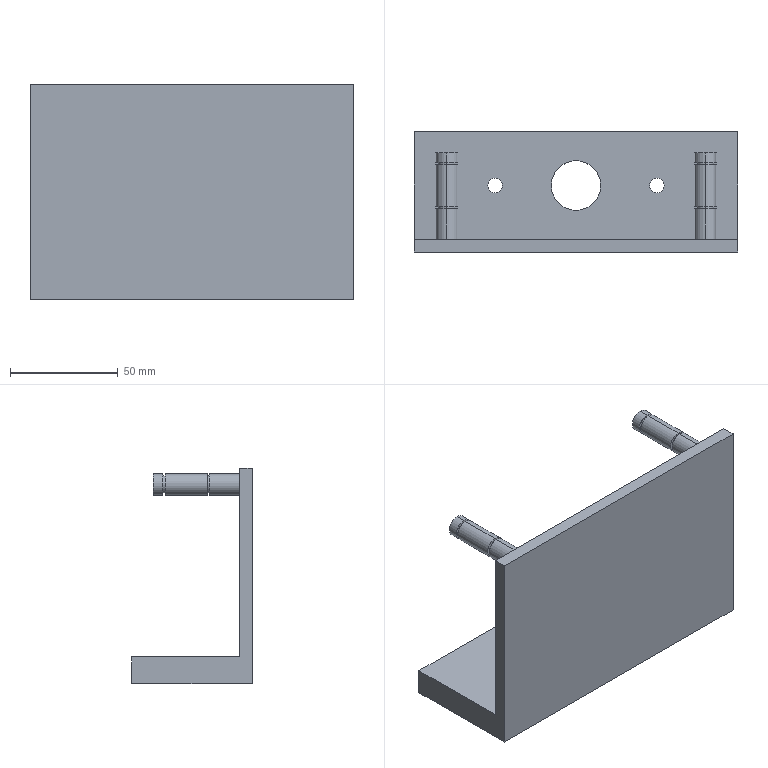Part | SolidWorks | features Cut 3, ICE 2, 3DProfileFeature 1, Extrusion 1, HoleWzd 1 | 1 solid | 44 faces | box 150 x 56 x 100 mm | volume 183819 mm3 | cylinder 26 | plane 18 | commonest cylinder face diameters 10 x12 8 x8 6.8 x4 23 x2
STEP:
#1=CARTESIAN_POINT('',(-60.,9.5,97.5));
#2=VERTEX_POINT('',#1);
#3=CARTESIAN_POINT('',(-60.,9.5,87.5));
#4=VERTEX_POINT('',#3);
#5=CARTESIAN_POINT('',(-60.,9.5,92.5));
#6=DIRECTION('',(0.,1.,0.));
#7=DIRECTION('',(0.,0.,1.));
#8=AXIS2_PLACEMENT_3D('',#5,#6,#7);
#9=CIRCLE('',#8,5.);
#10=EDGE_CURVE('',#2,#4,#9,.T.);
#11=ORIENTED_EDGE('',*,*,#10,.F.);
#12=CARTESIAN_POINT('',(-60.,-10.,97.5));
#13=VERTEX_POINT('',#12);
#14=CARTESIAN_POINT('',(-60.,15.,97.5));
#15=DIRECTION('',(0.,-1.,0.));
#16=VECTOR('',#15,1000.);
#17=LINE('',#14,#16);
#18=EDGE_CURVE('',#2,#13,#17,.T.);
#19=ORIENTED_EDGE('',*,*,#18,.T.);
#20=CARTESIAN_POINT('',(-60.,-10.,87.5));
#21=VERTEX_POINT('',#20);
#22=CARTESIAN_POINT('',(-60.,-10.,92.5));
#23=DIRECTION('',(0.,1.,0.));
#24=DIRECTION('',(0.,0.,1.));
#25=AXIS2_PLACEMENT_3D('',#22,#23,#24);
#26=CIRCLE('',#25,5.);
#27=EDGE_CURVE('',#13,#21,#26,.T.);
#28=ORIENTED_EDGE('',*,*,#27,.T.);
#29=CARTESIAN_POINT('',(-60.,15.,87.5));
#30=DIRECTION('',(0.,-1.,0.));
#31=VECTOR('',#30,1000.);
#32=LINE('',#29,#31);
#33=EDGE_CURVE('',#4,#21,#32,.T.);
#34=ORIENTED_EDGE('',*,*,#33,.F.);
#35=EDGE_LOOP('',(#11,#19,#28,#34));
#36=FACE_OUTER_BOUND('',#35,.T.);
#37=CARTESIAN_POINT('',(-60.,15.,92.5));
#38=DIRECTION('',(0.,-1.,0.));
#39=DIRECTION('',(0.,0.,-1.));
#40=AXIS2_PLACEMENT_3D('',#37,#38,#39);
#41=CYLINDRICAL_SURFACE('',#40,5.);
#42=ADVANCED_FACE('',(#36),#41,.T.);
#43=CARTESIAN_POINT('',(-60.,9.5,96.5));
#44=VERTEX_POINT('',#43);
#45=CARTESIAN_POINT('',(-60.,9.5,88.5));
#46=VERTEX_POINT('',#45);
#47=CARTESIAN_POINT('',(-60.,9.5,92.5));
#48=DIRECTION('',(0.,1.,0.));
#49=DIRECTION('',(0.,0.,1.));
#50=AXIS2_PLACEMENT_3D('',#47,#48,#49);
#51=CIRCLE('',#50,4.);
#52=EDGE_CURVE('',#44,#46,#51,.T.);
#53=ORIENTED_EDGE('',*,*,#52,.T.);
#54=CARTESIAN_POINT('',(-60.,10.5,88.5));
#55=VERTEX_POINT('',#54);
#56=CARTESIAN_POINT('',(-60.,9.5,88.5));
#57=DIRECTION('',(0.,1.,0.));
#58=VECTOR('',#57,1000.);
#59=LINE('',#56,#58);
#60=EDGE_CURVE('',#46,#55,#59,.T.);
#61=ORIENTED_EDGE('',*,*,#60,.T.);
#62=CARTESIAN_POINT('',(-60.,10.5,96.5));
#63=VERTEX_POINT('',#62);
#64=CARTESIAN_POINT('',(-60.,10.5,92.5));
#65=DIRECTION('',(0.,1.,0.));
#66=DIRECTION('',(0.,0.,1.));
#67=AXIS2_PLACEMENT_3D('',#64,#65,#66);
#68=CIRCLE('',#67,4.);
#69=EDGE_CURVE('',#63,#55,#68,.T.);
#70=ORIENTED_EDGE('',*,*,#69,.F.);
#71=CARTESIAN_POINT('',(-60.,9.5,96.5));
#72=DIRECTION('',(0.,1.,0.));
#73=VECTOR('',#72,1000.);
#74=LINE('',#71,#73);
#75=EDGE_CURVE('',#44,#63,#74,.T.);
#76=ORIENTED_EDGE('',*,*,#75,.F.);
#77=EDGE_LOOP('',(#53,#61,#70,#76));
#78=FACE_OUTER_BOUND('',#77,.T.);
#79=CARTESIAN_POINT('',(-60.,9.5,92.5));
#80=DIRECTION('',(0.,1.,0.));
#81=DIRECTION('',(0.,0.,1.));
#82=AXIS2_PLACEMENT_3D('',#79,#80,#81);
#83=CYLINDRICAL_SURFACE('',#82,4.);
#84=ADVANCED_FACE('',(#78),#83,.T.);
#85=CARTESIAN_POINT('',(-60.,15.,97.5));
#86=VERTEX_POINT('',#85);
#87=CARTESIAN_POINT('',(-60.,15.,87.5));
#88=VERTEX_POINT('',#87);
#89=CARTESIAN_POINT('',(-60.,15.,92.5));
#90=DIRECTION('',(0.,1.,0.));
#91=DIRECTION('',(0.,0.,1.));
#92=AXIS2_PLACEMENT_3D('',#89,#90,#91);
#93=CIRCLE('',#92,5.);
#94=EDGE_CURVE('',#86,#88,#93,.T.);
#95=ORIENTED_EDGE('',*,*,#94,.F.);
#96=CARTESIAN_POINT('',(-60.,10.5,97.5));
#97=VERTEX_POINT('',#96);
#98=CARTESIAN_POINT('',(-60.,15.,97.5));
#99=DIRECTION('',(0.,-1.,0.));
#100=VECTOR('',#99,1000.);
#101=LINE('',#98,#100);
#102=EDGE_CURVE('',#86,#97,#101,.T.);
#103=ORIENTED_EDGE('',*,*,#102,.T.);
#104=CARTESIAN_POINT('',(-60.,10.5,87.5));
#105=VERTEX_POINT('',#104);
#106=CARTESIAN_POINT('',(-60.,10.5,92.5));
#107=DIRECTION('',(0.,1.,0.));
#108=DIRECTION('',(0.,0.,1.));
#109=AXIS2_PLACEMENT_3D('',#106,#107,#108);
#110=CIRCLE('',#109,5.);
#111=EDGE_CURVE('',#97,#105,#110,.T.);
#112=ORIENTED_EDGE('',*,*,#111,.T.);
#113=CARTESIAN_POINT('',(-60.,15.,87.5));
#114=DIRECTION('',(0.,-1.,0.));
#115=VECTOR('',#114,1000.);
#116=LINE('',#113,#115);
#117=EDGE_CURVE('',#88,#105,#116,.T.);
#118=ORIENTED_EDGE('',*,*,#117,.F.);
#119=EDGE_LOOP('',(#95,#103,#112,#118));
#120=FACE_OUTER_BOUND('',#119,.T.);
#121=CARTESIAN_POINT('',(-60.,15.,92.5));
#122=DIRECTION('',(0.,-1.,0.));
#123=DIRECTION('',(0.,0.,-1.));
#124=AXIS2_PLACEMENT_3D('',#121,#122,#123);
#125=CYLINDRICAL_SURFACE('',#124,5.);
#126=ADVANCED_FACE('',(#120),#125,.T.);
#127=CARTESIAN_POINT('',(-60.,-11.,96.5));
#128=VERTEX_POINT('',#127);
#129=CARTESIAN_POINT('',(-60.,-11.,88.5));
#130=VERTEX_POINT('',#129);
#131=CARTESIAN_POINT('',(-60.,-11.,92.5));
#132=DIRECTION('',(0.,1.,0.));
#133=DIRECTION('',(0.,0.,1.));
#134=AXIS2_PLACEMENT_3D('',#131,#132,#133);
#135=CIRCLE('',#134,4.);
#136=EDGE_CURVE('',#128,#130,#135,.T.);
#137=ORIENTED_EDGE('',*,*,#136,.T.);
#138=CARTESIAN_POINT('',(-60.,-10.,88.5));
#139=VERTEX_POINT('',#138);
#140=CARTESIAN_POINT('',(-60.,-11.,88.5));
#141=DIRECTION('',(0.,1.,0.));
#142=VECTOR('',#141,1000.);
#143=LINE('',#140,#142);
#144=EDGE_CURVE('',#130,#139,#143,.T.);
#145=ORIENTED_EDGE('',*,*,#144,.T.);
#146=CARTESIAN_POINT('',(-60.,-10.,96.5));
#147=VERTEX_POINT('',#146);
#148=CARTESIAN_POINT('',(-60.,-10.,92.5));
#149=DIRECTION('',(0.,1.,0.));
#150=DIRECTION('',(0.,0.,1.));
#151=AXIS2_PLACEMENT_3D('',#148,#149,#150);
#152=CIRCLE('',#151,4.);
#153=EDGE_CURVE('',#147,#139,#152,.T.);
#154=ORIENTED_EDGE('',*,*,#153,.F.);
#155=CARTESIAN_POINT('',(-60.,-11.,96.5));
#156=DIRECTION('',(0.,1.,0.));
#157=VECTOR('',#156,1000.);
#158=LINE('',#155,#157);
#159=EDGE_CURVE('',#128,#147,#158,.T.);
#160=ORIENTED_EDGE('',*,*,#159,.F.);
#161=EDGE_LOOP('',(#137,#145,#154,#160));
#162=FACE_OUTER_BOUND('',#161,.T.);
#163=CARTESIAN_POINT('',(-60.,-11.,92.5));
#164=DIRECTION('',(0.,1.,0.));
#165=DIRECTION('',(0.,0.,1.));
#166=AXIS2_PLACEMENT_3D('',#163,#164,#165);
#167=CYLINDRICAL_SURFACE('',#166,4.);
#168=ADVANCED_FACE('',(#162),#167,.T.);
#169=CARTESIAN_POINT('',(60.,9.5,97.5));
#170=VERTEX_POINT('',#169);
#171=CARTESIAN_POINT('',(60.,9.5,87.5));
#172=VERTEX_POINT('',#171);
#173=CARTESIAN_POINT('',(60.,9.5,92.5));
#174=DIRECTION('',(0.,1.,0.));
#175=DIRECTION('',(0.,0.,1.));
#176=AXIS2_PLACEMENT_3D('',#173,#174,#175);
#177=CIRCLE('',#176,5.);
#178=EDGE_CURVE('',#170,#172,#177,.T.);
#179=ORIENTED_EDGE('',*,*,#178,.F.);
#180=CARTESIAN_POINT('',(60.,-10.,97.5));
#181=VERTEX_POINT('',#180);
#182=CARTESIAN_POINT('',(60.,15.,97.5));
#183=DIRECTION('',(0.,-1.,0.));
#184=VECTOR('',#183,1000.);
#185=LINE('',#182,#184);
#186=EDGE_CURVE('',#170,#181,#185,.T.);
#187=ORIENTED_EDGE('',*,*,#186,.T.);
#188=CARTESIAN_POINT('',(60.,-10.,87.5));
#189=VERTEX_POINT('',#188);
#190=CARTESIAN_POINT('',(60.,-10.,92.5));
#191=DIRECTION('',(0.,1.,0.));
#192=DIRECTION('',(0.,0.,1.));
#193=AXIS2_PLACEMENT_3D('',#190,#191,#192);
#194=CIRCLE('',#193,5.);
#195=EDGE_CURVE('',#181,#189,#194,.T.);
#196=ORIENTED_EDGE('',*,*,#195,.T.);
#197=CARTESIAN_POINT('',(60.,15.,87.5));
#198=DIRECTION('',(0.,-1.,0.));
#199=VECTOR('',#198,1000.);
#200=LINE('',#197,#199);
#201=EDGE_CURVE('',#172,#189,#200,.T.);
#202=ORIENTED_EDGE('',*,*,#201,.F.);
#203=EDGE_LOOP('',(#179,#187,#196,#202));
#204=FACE_OUTER_BOUND('',#203,.T.);
#205=CARTESIAN_POINT('',(60.,15.,92.5));
#206=DIRECTION('',(0.,-1.,0.));
#207=DIRECTION('',(0.,0.,-1.));
#208=AXIS2_PLACEMENT_3D('',#205,#206,#207);
#209=CYLINDRICAL_SURFACE('',#208,5.);
#210=ADVANCED_FACE('',(#204),#209,.T.);
#211=CARTESIAN_POINT('',(60.,9.5,96.5));
#212=VERTEX_POINT('',#211);
#213=CARTESIAN_POINT('',(60.,9.5,88.5));
#214=VERTEX_POINT('',#213);
#215=CARTESIAN_POINT('',(60.,9.5,92.5));
#216=DIRECTION('',(0.,1.,0.));
#217=DIRECTION('',(0.,0.,1.));
#218=AXIS2_PLACEMENT_3D('',#215,#216,#217);
#219=CIRCLE('',#218,4.);
#220=EDGE_CURVE('',#212,#214,#219,.T.);
#221=ORIENTED_EDGE('',*,*,#220,.T.);
#222=CARTESIAN_POINT('',(60.,10.5,88.5));
#223=VERTEX_POINT('',#222);
#224=CARTESIAN_POINT('',(60.,9.5,88.5));
#225=DIRECTION('',(0.,1.,0.));
#226=VECTOR('',#225,1000.);
#227=LINE('',#224,#226);
#228=EDGE_CURVE('',#214,#223,#227,.T.);
#229=ORIENTED_EDGE('',*,*,#228,.T.);
#230=CARTESIAN_POINT('',(60.,10.5,96.5));
#231=VERTEX_POINT('',#230);
#232=CARTESIAN_POINT('',(60.,10.5,92.5));
#233=DIRECTION('',(0.,1.,0.));
#234=DIRECTION('',(0.,0.,1.));
#235=AXIS2_PLACEMENT_3D('',#232,#233,#234);
#236=CIRCLE('',#235,4.);
#237=EDGE_CURVE('',#231,#223,#236,.T.);
#238=ORIENTED_EDGE('',*,*,#237,.F.);
#239=CARTESIAN_POINT('',(60.,9.5,96.5));
#240=DIRECTION('',(0.,1.,0.));
#241=VECTOR('',#240,1000.);
#242=LINE('',#239,#241);
#243=EDGE_CURVE('',#212,#231,#242,.T.);
#244=ORIENTED_EDGE('',*,*,#243,.F.);
#245=EDGE_LOOP('',(#221,#229,#238,#244));
#246=FACE_OUTER_BOUND('',#245,.T.);
#247=CARTESIAN_POINT('',(60.,9.5,92.5));
#248=DIRECTION('',(0.,1.,0.));
#249=DIRECTION('',(0.,0.,1.));
#250=AXIS2_PLACEMENT_3D('',#247,#248,#249);
#251=CYLINDRICAL_SURFACE('',#250,4.);
#252=ADVANCED_FACE('',(#246),#251,.T.);
#253=CARTESIAN_POINT('',(60.,15.,97.5));
#254=VERTEX_POINT('',#253);
#255=CARTESIAN_POINT('',(60.,15.,87.5));
#256=VERTEX_POINT('',#255);
#257=CARTESIAN_POINT('',(60.,15.,92.5));
#258=DIRECTION('',(0.,1.,0.));
#259=DIRECTION('',(0.,0.,1.));
#260=AXIS2_PLACEMENT_3D('',#257,#258,#259);
#261=CIRCLE('',#260,5.);
#262=EDGE_CURVE('',#254,#256,#261,.T.);
#263=ORIENTED_EDGE('',*,*,#262,.F.);
#264=CARTESIAN_POINT('',(60.,10.5,97.5));
#265=VERTEX_POINT('',#264);
#266=CARTESIAN_POINT('',(60.,15.,97.5));
#267=DIRECTION('',(0.,-1.,0.));
#268=VECTOR('',#267,1000.);
#269=LINE('',#266,#268);
#270=EDGE_CURVE('',#254,#265,#269,.T.);
#271=ORIENTED_EDGE('',*,*,#270,.T.);
#272=CARTESIAN_POINT('',(60.,10.5,87.5));
#273=VERTEX_POINT('',#272);
#274=CARTESIAN_POINT('',(60.,10.5,92.5));
#275=DIRECTION('',(0.,1.,0.));
#276=DIRECTION('',(0.,0.,1.));
#277=AXIS2_PLACEMENT_3D('',#274,#275,#276);
#278=CIRCLE('',#277,5.);
#279=EDGE_CURVE('',#265,#273,#278,.T.);
#280=ORIENTED_EDGE('',*,*,#279,.T.);
#281=CARTESIAN_POINT('',(60.,15.,87.5));
#282=DIRECTION('',(0.,-1.,0.));
#283=VECTOR('',#282,1000.);
#284=LINE('',#281,#283);
#285=EDGE_CURVE('',#256,#273,#284,.T.);
#286=ORIENTED_EDGE('',*,*,#285,.F.);
#287=EDGE_LOOP('',(#263,#271,#280,#286));
#288=FACE_OUTER_BOUND('',#287,.T.);
#289=CARTESIAN_POINT('',(60.,15.,92.5));
#290=DIRECTION('',(0.,-1.,0.));
#291=DIRECTION('',(0.,0.,-1.));
#292=AXIS2_PLACEMENT_3D('',#289,#290,#291);
#293=CYLINDRICAL_SURFACE('',#292,5.);
#294=ADVANCED_FACE('',(#288),#293,.T.);
#295=CARTESIAN_POINT('',(60.,-11.,96.5));
#296=VERTEX_POINT('',#295);
#297=CARTESIAN_POINT('',(60.,-11.,88.5));
#298=VERTEX_POINT('',#297);
#299=CARTESIAN_POINT('',(60.,-11.,92.5));
#300=DIRECTION('',(0.,1.,0.));
#301=DIRECTION('',(0.,0.,1.));
#302=AXIS2_PLACEMENT_3D('',#299,#300,#301);
#303=CIRCLE('',#302,4.);
#304=EDGE_CURVE('',#296,#298,#303,.T.);
#305=ORIENTED_EDGE('',*,*,#304,.T.);
#306=CARTESIAN_POINT('',(60.,-10.,88.5));
#307=VERTEX_POINT('',#306);
#308=CARTESIAN_POINT('',(60.,-11.,88.5));
#309=DIRECTION('',(0.,1.,0.));
#310=VECTOR('',#309,1000.);
#311=LINE('',#308,#310);
#312=EDGE_CURVE('',#298,#307,#311,.T.);
#313=ORIENTED_EDGE('',*,*,#312,.T.);
#314=CARTESIAN_POINT('',(60.,-10.,96.5));
#315=VERTEX_POINT('',#314);
#316=CARTESIAN_POINT('',(60.,-10.,92.5));
#317=DIRECTION('',(0.,1.,0.));
#318=DIRECTION('',(0.,0.,1.));
#319=AXIS2_PLACEMENT_3D('',#316,#317,#318);
#320=CIRCLE('',#319,4.);
#321=EDGE_CURVE('',#315,#307,#320,.T.);
#322=ORIENTED_EDGE('',*,*,#321,.F.);
#323=CARTESIAN_POINT('',(60.,-11.,96.5));
#324=DIRECTION('',(0.,1.,0.));
#325=VECTOR('',#324,1000.);
#326=LINE('',#323,#325);
#327=EDGE_CURVE('',#296,#315,#326,.T.);
#328=ORIENTED_EDGE('',*,*,#327,.F.);
#329=EDGE_LOOP('',(#305,#313,#322,#328));
#330=FACE_OUTER_BOUND('',#329,.T.);
#331=CARTESIAN_POINT('',(60.,-11.,92.5));
#332=DIRECTION('',(0.,1.,0.));
#333=DIRECTION('',(0.,0.,1.));
#334=AXIS2_PLACEMENT_3D('',#331,#332,#333);
#335=CYLINDRICAL_SURFACE('',#334,4.);
#336=ADVANCED_FACE('',(#330),#335,.T.);
#337=CARTESIAN_POINT('',(40.9,0.,12.5));
#338=VERTEX_POINT('',#337);
#339=CARTESIAN_POINT('',(34.1,0.,12.5));
#340=VERTEX_POINT('',#339);
#341=CARTESIAN_POINT('',(37.5,0.,12.5));
#342=DIRECTION('',(0.,0.,-1.));
#343=DIRECTION('',(-1.,0.,0.));
#344=AXIS2_PLACEMENT_3D('',#341,#342,#343);
#345=CIRCLE('',#344,3.4);
#346=EDGE_CURVE('',#338,#340,#345,.T.);
#347=ORIENTED_EDGE('',*,*,#346,.F.);
#348=CARTESIAN_POINT('',(40.9,0.,0.));
#349=VERTEX_POINT('',#348);
#350=CARTESIAN_POINT('',(40.9,0.,0.));
#351=DIRECTION('',(0.,0.,-1.));
#352=VECTOR('',#351,1000.);
#353=LINE('',#350,#352);
#354=EDGE_CURVE('',#338,#349,#353,.T.);
#355=ORIENTED_EDGE('',*,*,#354,.T.);
#356=CARTESIAN_POINT('',(34.1,0.,0.));
#357=VERTEX_POINT('',#356);
#358=CARTESIAN_POINT('',(37.5,0.,0.));
#359=DIRECTION('',(0.,0.,-1.));
#360=DIRECTION('',(-1.,0.,0.));
#361=AXIS2_PLACEMENT_3D('',#358,#359,#360);
#362=CIRCLE('',#361,3.4);
#363=EDGE_CURVE('',#349,#357,#362,.T.);
#364=ORIENTED_EDGE('',*,*,#363,.T.);
#365=CARTESIAN_POINT('',(34.1,0.,0.));
#366=DIRECTION('',(0.,0.,-1.));
#367=VECTOR('',#366,1000.);
#368=LINE('',#365,#367);
#369=EDGE_CURVE('',#340,#357,#368,.T.);
#370=ORIENTED_EDGE('',*,*,#369,.F.);
#371=EDGE_LOOP('',(#347,#355,#364,#370));
#372=FACE_OUTER_BOUND('',#371,.T.);
#373=CARTESIAN_POINT('',(37.5,0.,0.));
#374=DIRECTION('',(0.,0.,-1.));
#375=DIRECTION('',(-1.,0.,0.));
#376=AXIS2_PLACEMENT_3D('',#373,#374,#375);
#377=CYLINDRICAL_SURFACE('',#376,3.4);
#378=ADVANCED_FACE('',(#372),#377,.F.);
#379=CARTESIAN_POINT('',(-34.1,0.,12.5));
#380=VERTEX_POINT('',#379);
#381=CARTESIAN_POINT('',(-40.9,0.,12.5));
#382=VERTEX_POINT('',#381);
#383=CARTESIAN_POINT('',(-37.5,0.,12.5));
#384=DIRECTION('',(0.,0.,-1.));
#385=DIRECTION('',(-1.,0.,0.));
#386=AXIS2_PLACEMENT_3D('',#383,#384,#385);
#387=CIRCLE('',#386,3.4);
#388=EDGE_CURVE('',#380,#382,#387,.T.);
#389=ORIENTED_EDGE('',*,*,#388,.F.);
#390=CARTESIAN_POINT('',(-34.1,0.,0.));
#391=VERTEX_POINT('',#390);
#392=CARTESIAN_POINT('',(-34.1,0.,0.));
#393=DIRECTION('',(0.,0.,-1.));
#394=VECTOR('',#393,1000.);
#395=LINE('',#392,#394);
#396=EDGE_CURVE('',#380,#391,#395,.T.);
#397=ORIENTED_EDGE('',*,*,#396,.T.);
#398=CARTESIAN_POINT('',(-40.9,0.,0.));
#399=VERTEX_POINT('',#398);
#400=CARTESIAN_POINT('',(-37.5,0.,0.));
#401=DIRECTION('',(0.,0.,-1.));
#402=DIRECTION('',(-1.,0.,0.));
#403=AXIS2_PLACEMENT_3D('',#400,#401,#402);
#404=CIRCLE('',#403,3.4);
#405=EDGE_CURVE('',#391,#399,#404,.T.);
#406=ORIENTED_EDGE('',*,*,#405,.T.);
#407=CARTESIAN_POINT('',(-40.9,0.,0.));
#408=DIRECTION('',(0.,0.,-1.));
#409=VECTOR('',#408,1000.);
#410=LINE('',#407,#409);
#411=EDGE_CURVE('',#382,#399,#410,.T.);
#412=ORIENTED_EDGE('',*,*,#411,.F.);
#413=EDGE_LOOP('',(#389,#397,#406,#412));
#414=FACE_OUTER_BOUND('',#413,.T.);
#415=CARTESIAN_POINT('',(-37.5,0.,0.));
#416=DIRECTION('',(0.,0.,-1.));
#417=DIRECTION('',(-1.,0.,0.));
#418=AXIS2_PLACEMENT_3D('',#415,#416,#417);
#419=CYLINDRICAL_SURFACE('',#418,3.4);
#420=ADVANCED_FACE('',(#414),#419,.F.);
#421=CARTESIAN_POINT('',(-11.5,0.,12.5));
#422=VERTEX_POINT('',#421);
#423=CARTESIAN_POINT('',(11.5,0.,12.5));
#424=VERTEX_POINT('',#423);
#425=CARTESIAN_POINT('',(0.,0.,12.5));
#426=DIRECTION('',(0.,0.,1.));
#427=DIRECTION('',(1.,0.,0.));
#428=AXIS2_PLACEMENT_3D('',#425,#426,#427);
#429=CIRCLE('',#428,11.5);
#430=EDGE_CURVE('',#422,#424,#429,.T.);
#431=ORIENTED_EDGE('',*,*,#430,.T.);
#432=CARTESIAN_POINT('',(11.5,0.,0.));
#433=VERTEX_POINT('',#432);
#434=CARTESIAN_POINT('',(11.5,0.,12.5));
#435=DIRECTION('',(0.,0.,-1.));
#436=VECTOR('',#435,1000.);
#437=LINE('',#434,#436);
#438=EDGE_CURVE('',#424,#433,#437,.T.);
#439=ORIENTED_EDGE('',*,*,#438,.T.);
#440=CARTESIAN_POINT('',(-11.5,0.,0.));
#441=VERTEX_POINT('',#440);
#442=CARTESIAN_POINT('',(0.,0.,0.));
#443=DIRECTION('',(0.,0.,1.));
#444=DIRECTION('',(1.,0.,0.));
#445=AXIS2_PLACEMENT_3D('',#442,#443,#444);
#446=CIRCLE('',#445,11.5);
#447=EDGE_CURVE('',#441,#433,#446,.T.);
#448=ORIENTED_EDGE('',*,*,#447,.F.);
#449=CARTESIAN_POINT('',(-11.5,0.,12.5));
#450=DIRECTION('',(0.,0.,-1.));
#451=VECTOR('',#450,1000.);
#452=LINE('',#449,#451);
#453=EDGE_CURVE('',#422,#441,#452,.T.);
#454=ORIENTED_EDGE('',*,*,#453,.F.);
#455=EDGE_LOOP('',(#431,#439,#448,#454));
#456=FACE_OUTER_BOUND('',#455,.T.);
#457=CARTESIAN_POINT('',(0.,0.,12.5));
#458=DIRECTION('',(0.,0.,-1.));
#459=DIRECTION('',(-1.,0.,0.));
#460=AXIS2_PLACEMENT_3D('',#457,#458,#459);
#461=CYLINDRICAL_SURFACE('',#460,11.5);
#462=ADVANCED_FACE('',(#456),#461,.F.);
#463=CARTESIAN_POINT('',(60.,-11.,97.5));
#464=VERTEX_POINT('',#463);
#465=CARTESIAN_POINT('',(60.,-11.,87.5));
#466=VERTEX_POINT('',#465);
#467=CARTESIAN_POINT('',(60.,-11.,92.5));
#468=DIRECTION('',(0.,1.,0.));
#469=DIRECTION('',(0.,0.,1.));
#470=AXIS2_PLACEMENT_3D('',#467,#468,#469);
#471=CIRCLE('',#470,5.);
#472=EDGE_CURVE('',#464,#466,#471,.T.);
#473=ORIENTED_EDGE('',*,*,#472,.F.);
#474=CARTESIAN_POINT('',(60.,-25.,97.5));
#475=VERTEX_POINT('',#474);
#476=CARTESIAN_POINT('',(60.,15.,97.5));
#477=DIRECTION('',(0.,-1.,0.));
#478=VECTOR('',#477,1000.);
#479=LINE('',#476,#478);
#480=EDGE_CURVE('',#464,#475,#479,.T.);
#481=ORIENTED_EDGE('',*,*,#480,.T.);
#482=CARTESIAN_POINT('',(60.,-25.,87.5));
#483=VERTEX_POINT('',#482);
#484=CARTESIAN_POINT('',(60.,-25.,92.5));
#485=DIRECTION('',(0.,1.,0.));
#486=DIRECTION('',(0.,0.,1.));
#487=AXIS2_PLACEMENT_3D('',#484,#485,#486);
#488=CIRCLE('',#487,5.);
#489=EDGE_CURVE('',#475,#483,#488,.T.);
#490=ORIENTED_EDGE('',*,*,#489,.T.);
#491=CARTESIAN_POINT('',(60.,15.,87.5));
#492=DIRECTION('',(0.,-1.,0.));
#493=VECTOR('',#492,1000.);
#494=LINE('',#491,#493);
#495=EDGE_CURVE('',#466,#483,#494,.T.);
#496=ORIENTED_EDGE('',*,*,#495,.F.);
#497=EDGE_LOOP('',(#473,#481,#490,#496));
#498=FACE_OUTER_BOUND('',#497,.T.);
#499=CARTESIAN_POINT('',(60.,15.,92.5));
#500=DIRECTION('',(0.,-1.,0.));
#501=DIRECTION('',(0.,0.,-1.));
#502=AXIS2_PLACEMENT_3D('',#499,#500,#501);
#503=CYLINDRICAL_SURFACE('',#502,5.);
#504=ADVANCED_FACE('',(#498),#503,.T.);
#505=CARTESIAN_POINT('',(-60.,-11.,97.5));
#506=VERTEX_POINT('',#505);
#507=CARTESIAN_POINT('',(-60.,-11.,87.5));
#508=VERTEX_POINT('',#507);
#509=CARTESIAN_POINT('',(-60.,-11.,92.5));
#510=DIRECTION('',(0.,1.,0.));
#511=DIRECTION('',(0.,0.,1.));
#512=AXIS2_PLACEMENT_3D('',#509,#510,#511);
#513=CIRCLE('',#512,5.);
#514=EDGE_CURVE('',#506,#508,#513,.T.);
#515=ORIENTED_EDGE('',*,*,#514,.F.);
#516=CARTESIAN_POINT('',(-60.,-25.,97.5));
#517=VERTEX_POINT('',#516);
#518=CARTESIAN_POINT('',(-60.,15.,97.5));
#519=DIRECTION('',(0.,-1.,0.));
#520=VECTOR('',#519,1000.);
#521=LINE('',#518,#520);
#522=EDGE_CURVE('',#506,#517,#521,.T.);
#523=ORIENTED_EDGE('',*,*,#522,.T.);
#524=CARTESIAN_POINT('',(-60.,-25.,87.5));
#525=VERTEX_POINT('',#524);
#526=CARTESIAN_POINT('',(-60.,-25.,92.5));
#527=DIRECTION('',(0.,1.,0.));
#528=DIRECTION('',(0.,0.,1.));
#529=AXIS2_PLACEMENT_3D('',#526,#527,#528);
#530=CIRCLE('',#529,5.);
#531=EDGE_CURVE('',#517,#525,#530,.T.);
#532=ORIENTED_EDGE('',*,*,#531,.T.);
#533=CARTESIAN_POINT('',(-60.,15.,87.5));
#534=DIRECTION('',(0.,-1.,0.));
#535=VECTOR('',#534,1000.);
#536=LINE('',#533,#535);
#537=EDGE_CURVE('',#508,#525,#536,.T.);
#538=ORIENTED_EDGE('',*,*,#537,.F.);
#539=EDGE_LOOP('',(#515,#523,#532,#538));
#540=FACE_OUTER_BOUND('',#539,.T.);
#541=CARTESIAN_POINT('',(-60.,15.,92.5));
#542=DIRECTION('',(0.,-1.,0.));
#543=DIRECTION('',(0.,0.,-1.));
#544=AXIS2_PLACEMENT_3D('',#541,#542,#543);
#545=CYLINDRICAL_SURFACE('',#544,5.);
#546=ADVANCED_FACE('',(#540),#545,.T.);
#547=ORIENTED_EDGE('',*,*,#522,.F.);
#548=CARTESIAN_POINT('',(-60.,-11.,92.5));
#549=DIRECTION('',(0.,1.,0.));
#550=DIRECTION('',(0.,0.,1.));
#551=AXIS2_PLACEMENT_3D('',#548,#549,#550);
#552=CIRCLE('',#551,5.);
#553=EDGE_CURVE('',#508,#506,#552,.T.);
#554=ORIENTED_EDGE('',*,*,#553,.F.);
#555=ORIENTED_EDGE('',*,*,#537,.T.);
#556=CARTESIAN_POINT('',(-60.,-25.,92.5));
#557=DIRECTION('',(0.,1.,0.));
#558=DIRECTION('',(0.,0.,1.));
#559=AXIS2_PLACEMENT_3D('',#556,#557,#558);
#560=CIRCLE('',#559,5.);
#561=EDGE_CURVE('',#525,#517,#560,.T.);
#562=ORIENTED_EDGE('',*,*,#561,.T.);
#563=EDGE_LOOP('',(#547,#554,#555,#562));
#564=FACE_OUTER_BOUND('',#563,.T.);
#565=CARTESIAN_POINT('',(-60.,15.,92.5));
#566=DIRECTION('',(0.,-1.,0.));
#567=DIRECTION('',(0.,0.,-1.));
#568=AXIS2_PLACEMENT_3D('',#565,#566,#567);
#569=CYLINDRICAL_SURFACE('',#568,5.);
#570=ADVANCED_FACE('',(#564),#569,.T.);
#571=ORIENTED_EDGE('',*,*,#480,.F.);
#572=CARTESIAN_POINT('',(60.,-11.,92.5));
#573=DIRECTION('',(0.,1.,0.));
#574=DIRECTION('',(0.,0.,1.));
#575=AXIS2_PLACEMENT_3D('',#572,#573,#574);
#576=CIRCLE('',#575,5.);
#577=EDGE_CURVE('',#466,#464,#576,.T.);
#578=ORIENTED_EDGE('',*,*,#577,.F.);
#579=ORIENTED_EDGE('',*,*,#495,.T.);
#580=CARTESIAN_POINT('',(60.,-25.,92.5));
#581=DIRECTION('',(0.,1.,0.));
#582=DIRECTION('',(0.,0.,1.));
#583=AXIS2_PLACEMENT_3D('',#580,#581,#582);
#584=CIRCLE('',#583,5.);
#585=EDGE_CURVE('',#483,#475,#584,.T.);
#586=ORIENTED_EDGE('',*,*,#585,.T.);
#587=EDGE_LOOP('',(#571,#578,#579,#586));
#588=FACE_OUTER_BOUND('',#587,.T.);
#589=CARTESIAN_POINT('',(60.,15.,92.5));
#590=DIRECTION('',(0.,-1.,0.));
#591=DIRECTION('',(0.,0.,-1.));
#592=AXIS2_PLACEMENT_3D('',#589,#590,#591);
#593=CYLINDRICAL_SURFACE('',#592,5.);
#594=ADVANCED_FACE('',(#588),#593,.T.);
#595=CARTESIAN_POINT('',(-75.,-25.,12.5));
#596=VERTEX_POINT('',#595);
#597=CARTESIAN_POINT('',(-75.,-25.,100.));
#598=VERTEX_POINT('',#597);
#599=CARTESIAN_POINT('',(-75.,-25.,0.));
#600=DIRECTION('',(0.,0.,1.));
#601=VECTOR('',#600,1000.);
#602=LINE('',#599,#601);
#603=EDGE_CURVE('',#596,#598,#602,.T.);
#604=ORIENTED_EDGE('',*,*,#603,.T.);
#605=CARTESIAN_POINT('',(75.,-25.,100.));
#606=VERTEX_POINT('',#605);
#607=CARTESIAN_POINT('',(-100.,-25.,100.));
#608=DIRECTION('',(-1.,0.,0.));
#609=VECTOR('',#608,1000.);
#610=LINE('',#607,#609);
#611=EDGE_CURVE('',#606,#598,#610,.T.);
#612=ORIENTED_EDGE('',*,*,#611,.F.);
#613=CARTESIAN_POINT('',(75.,-25.,12.5));
#614=VERTEX_POINT('',#613);
#615=CARTESIAN_POINT('',(75.,-25.,0.));
#616=DIRECTION('',(0.,0.,-1.));
#617=VECTOR('',#616,1000.);
#618=LINE('',#615,#617);
#619=EDGE_CURVE('',#606,#614,#618,.T.);
#620=ORIENTED_EDGE('',*,*,#619,.T.);
#621=CARTESIAN_POINT('',(-100.,-25.,12.5));
#622=DIRECTION('',(1.,0.,0.));
#623=VECTOR('',#622,1000.);
#624=LINE('',#621,#623);
#625=EDGE_CURVE('',#596,#614,#624,.T.);
#626=ORIENTED_EDGE('',*,*,#625,.F.);
#627=EDGE_LOOP('',(#604,#612,#620,#626));
#628=FACE_OUTER_BOUND('',#627,.T.);
#629=ORIENTED_EDGE('',*,*,#585,.F.);
#630=ORIENTED_EDGE('',*,*,#489,.F.);
#631=EDGE_LOOP('',(#629,#630));
#632=FACE_BOUND('',#631,.T.);
#633=ORIENTED_EDGE('',*,*,#561,.F.);
#634=ORIENTED_EDGE('',*,*,#531,.F.);
#635=EDGE_LOOP('',(#633,#634));
#636=FACE_BOUND('',#635,.T.);
#637=CARTESIAN_POINT('',(0.,-25.,0.));
#638=DIRECTION('',(0.,1.,0.));
#639=DIRECTION('',(0.,0.,1.));
#640=AXIS2_PLACEMENT_3D('',#637,#638,#639);
#641=PLANE('',#640);
#642=ADVANCED_FACE('',(#628,#632,#636),#641,.T.);
#643=CARTESIAN_POINT('',(37.5,0.,12.5));
#644=DIRECTION('',(0.,0.,-1.));
#645=DIRECTION('',(-1.,0.,0.));
#646=AXIS2_PLACEMENT_3D('',#643,#644,#645);
#647=CIRCLE('',#646,3.4);
#648=EDGE_CURVE('',#340,#338,#647,.T.);
#649=ORIENTED_EDGE('',*,*,#648,.T.);
#650=ORIENTED_EDGE('',*,*,#346,.T.);
#651=EDGE_LOOP('',(#649,#650));
#652=FACE_BOUND('',#651,.T.);
#653=CARTESIAN_POINT('',(-37.5,0.,12.5));
#654=DIRECTION('',(0.,0.,-1.));
#655=DIRECTION('',(-1.,0.,0.));
#656=AXIS2_PLACEMENT_3D('',#653,#654,#655);
#657=CIRCLE('',#656,3.4);
#658=EDGE_CURVE('',#382,#380,#657,.T.);
#659=ORIENTED_EDGE('',*,*,#658,.T.);
#660=ORIENTED_EDGE('',*,*,#388,.T.);
#661=EDGE_LOOP('',(#659,#660));
#662=FACE_BOUND('',#661,.T.);
#663=CARTESIAN_POINT('',(75.,25.,12.5));
#664=VERTEX_POINT('',#663);
#665=CARTESIAN_POINT('',(-75.,25.,12.5));
#666=VERTEX_POINT('',#665);
#667=CARTESIAN_POINT('',(-100.,25.,12.5));
#668=DIRECTION('',(-1.,0.,0.));
#669=VECTOR('',#668,1000.);
#670=LINE('',#667,#669);
#671=EDGE_CURVE('',#664,#666,#670,.T.);
#672=ORIENTED_EDGE('',*,*,#671,.T.);
#673=CARTESIAN_POINT('',(-75.,25.001,12.5));
#674=DIRECTION('',(0.,1.,0.));
#675=VECTOR('',#674,1000.);
#676=LINE('',#673,#675);
#677=EDGE_CURVE('',#596,#666,#676,.T.);
#678=ORIENTED_EDGE('',*,*,#677,.F.);
#679=ORIENTED_EDGE('',*,*,#625,.T.);
#680=CARTESIAN_POINT('',(75.,25.001,12.5));
#681=DIRECTION('',(0.,-1.,0.));
#682=VECTOR('',#681,1000.);
#683=LINE('',#680,#682);
#684=EDGE_CURVE('',#664,#614,#683,.T.);
#685=ORIENTED_EDGE('',*,*,#684,.F.);
#686=EDGE_LOOP('',(#672,#678,#679,#685));
#687=FACE_OUTER_BOUND('',#686,.T.);
#688=ORIENTED_EDGE('',*,*,#430,.F.);
#689=CARTESIAN_POINT('',(0.,0.,12.5));
#690=DIRECTION('',(0.,0.,1.));
#691=DIRECTION('',(1.,0.,0.));
#692=AXIS2_PLACEMENT_3D('',#689,#690,#691);
#693=CIRCLE('',#692,11.5);
#694=EDGE_CURVE('',#424,#422,#693,.T.);
#695=ORIENTED_EDGE('',*,*,#694,.F.);
#696=EDGE_LOOP('',(#688,#695));
#697=FACE_BOUND('',#696,.T.);
#698=CARTESIAN_POINT('',(0.,0.,12.5));
#699=DIRECTION('',(0.,0.,-1.));
#700=DIRECTION('',(-1.,0.,0.));
#701=AXIS2_PLACEMENT_3D('',#698,#699,#700);
#702=PLANE('',#701);
#703=ADVANCED_FACE('',(#652,#662,#687,#697),#702,.F.);
#704=CARTESIAN_POINT('',(-75.,25.,0.));
#705=VERTEX_POINT('',#704);
#706=CARTESIAN_POINT('',(-75.,-31.,0.));
#707=VERTEX_POINT('',#706);
#708=CARTESIAN_POINT('',(-75.,25.001,0.));
#709=DIRECTION('',(0.,-1.,0.));
#710=VECTOR('',#709,1000.);
#711=LINE('',#708,#710);
#712=EDGE_CURVE('',#705,#707,#711,.T.);
#713=ORIENTED_EDGE('',*,*,#712,.F.);
#714=CARTESIAN_POINT('',(75.,25.,0.));
#715=VERTEX_POINT('',#714);
#716=CARTESIAN_POINT('',(-100.,25.,0.));
#717=DIRECTION('',(-1.,0.,0.));
#718=VECTOR('',#717,1000.);
#719=LINE('',#716,#718);
#720=EDGE_CURVE('',#715,#705,#719,.T.);
#721=ORIENTED_EDGE('',*,*,#720,.F.);
#722=CARTESIAN_POINT('',(75.,-31.,0.));
#723=VERTEX_POINT('',#722);
#724=CARTESIAN_POINT('',(75.,25.001,0.));
#725=DIRECTION('',(0.,-1.,0.));
#726=VECTOR('',#725,1000.);
#727=LINE('',#724,#726);
#728=EDGE_CURVE('',#715,#723,#727,.T.);
#729=ORIENTED_EDGE('',*,*,#728,.T.);
#730=CARTESIAN_POINT('',(-100.,-31.,0.));
#731=DIRECTION('',(1.,0.,0.));
#732=VECTOR('',#731,1000.);
#733=LINE('',#730,#732);
#734=EDGE_CURVE('',#707,#723,#733,.T.);
#735=ORIENTED_EDGE('',*,*,#734,.F.);
#736=EDGE_LOOP('',(#713,#721,#729,#735));
#737=FACE_OUTER_BOUND('',#736,.T.);
#738=CARTESIAN_POINT('',(37.5,0.,0.));
#739=DIRECTION('',(0.,0.,-1.));
#740=DIRECTION('',(-1.,0.,0.));
#741=AXIS2_PLACEMENT_3D('',#738,#739,#740);
#742=CIRCLE('',#741,3.4);
#743=EDGE_CURVE('',#357,#349,#742,.T.);
#744=ORIENTED_EDGE('',*,*,#743,.F.);
#745=ORIENTED_EDGE('',*,*,#363,.F.);
#746=EDGE_LOOP('',(#744,#745));
#747=FACE_BOUND('',#746,.T.);
#748=CARTESIAN_POINT('',(-37.5,0.,0.));
#749=DIRECTION('',(0.,0.,-1.));
#750=DIRECTION('',(-1.,0.,0.));
#751=AXIS2_PLACEMENT_3D('',#748,#749,#750);
#752=CIRCLE('',#751,3.4);
#753=EDGE_CURVE('',#399,#391,#752,.T.);
#754=ORIENTED_EDGE('',*,*,#753,.F.);
#755=ORIENTED_EDGE('',*,*,#405,.F.);
#756=EDGE_LOOP('',(#754,#755));
#757=FACE_BOUND('',#756,.T.);
#758=ORIENTED_EDGE('',*,*,#447,.T.);
#759=CARTESIAN_POINT('',(0.,0.,0.));
#760=DIRECTION('',(0.,0.,1.));
#761=DIRECTION('',(1.,0.,0.));
#762=AXIS2_PLACEMENT_3D('',#759,#760,#761);
#763=CIRCLE('',#762,11.5);
#764=EDGE_CURVE('',#433,#441,#763,.T.);
#765=ORIENTED_EDGE('',*,*,#764,.T.);
#766=EDGE_LOOP('',(#758,#765));
#767=FACE_BOUND('',#766,.T.);
#768=CARTESIAN_POINT('',(0.,0.,0.));
#769=DIRECTION('',(0.,0.,-1.));
#770=DIRECTION('',(-1.,0.,0.));
#771=AXIS2_PLACEMENT_3D('',#768,#769,#770);
#772=PLANE('',#771);
#773=ADVANCED_FACE('',(#737,#747,#757,#767),#772,.T.);
#774=ORIENTED_EDGE('',*,*,#720,.T.);
#775=CARTESIAN_POINT('',(-75.,25.,0.));
#776=DIRECTION('',(0.,0.,-1.));
#777=VECTOR('',#776,1000.);
#778=LINE('',#775,#777);
#779=EDGE_CURVE('',#666,#705,#778,.T.);
#780=ORIENTED_EDGE('',*,*,#779,.F.);
#781=ORIENTED_EDGE('',*,*,#671,.F.);
#782=CARTESIAN_POINT('',(75.,25.,0.));
#783=DIRECTION('',(0.,0.,1.));
#784=VECTOR('',#783,1000.);
#785=LINE('',#782,#784);
#786=EDGE_CURVE('',#715,#664,#785,.T.);
#787=ORIENTED_EDGE('',*,*,#786,.F.);
#788=EDGE_LOOP('',(#774,#780,#781,#787));
#789=FACE_OUTER_BOUND('',#788,.T.);
#790=CARTESIAN_POINT('',(-100.,25.,12.5));
#791=DIRECTION('',(0.,-1.,0.));
#792=DIRECTION('',(0.,0.,-1.));
#793=AXIS2_PLACEMENT_3D('',#790,#791,#792);
#794=PLANE('',#793);
#795=ADVANCED_FACE('',(#789),#794,.F.);
#796=ORIENTED_EDGE('',*,*,#438,.F.);
#797=ORIENTED_EDGE('',*,*,#694,.T.);
#798=ORIENTED_EDGE('',*,*,#453,.T.);
#799=ORIENTED_EDGE('',*,*,#764,.F.);
#800=EDGE_LOOP('',(#796,#797,#798,#799));
#801=FACE_OUTER_BOUND('',#800,.T.);
#802=CARTESIAN_POINT('',(0.,0.,12.5));
#803=DIRECTION('',(0.,0.,-1.));
#804=DIRECTION('',(-1.,0.,0.));
#805=AXIS2_PLACEMENT_3D('',#802,#803,#804);
#806=CYLINDRICAL_SURFACE('',#805,11.5);
#807=ADVANCED_FACE('',(#801),#806,.F.);
#808=ORIENTED_EDGE('',*,*,#611,.T.);
#809=CARTESIAN_POINT('',(-75.,-31.,100.));
#810=VERTEX_POINT('',#809);
#811=CARTESIAN_POINT('',(-75.,25.001,100.));
#812=DIRECTION('',(0.,-1.,0.));
#813=VECTOR('',#812,1000.);
#814=LINE('',#811,#813);
#815=EDGE_CURVE('',#598,#810,#814,.T.);
#816=ORIENTED_EDGE('',*,*,#815,.T.);
#817=CARTESIAN_POINT('',(75.,-31.,100.));
#818=VERTEX_POINT('',#817);
#819=CARTESIAN_POINT('',(-100.,-31.,100.));
#820=DIRECTION('',(-1.,0.,0.));
#821=VECTOR('',#820,1000.);
#822=LINE('',#819,#821);
#823=EDGE_CURVE('',#818,#810,#822,.T.);
#824=ORIENTED_EDGE('',*,*,#823,.F.);
#825=CARTESIAN_POINT('',(75.,25.001,100.));
#826=DIRECTION('',(0.,-1.,0.));
#827=VECTOR('',#826,1000.);
#828=LINE('',#825,#827);
#829=EDGE_CURVE('',#606,#818,#828,.T.);
#830=ORIENTED_EDGE('',*,*,#829,.F.);
#831=EDGE_LOOP('',(#808,#816,#824,#830));
#832=FACE_OUTER_BOUND('',#831,.T.);
#833=CARTESIAN_POINT('',(-100.,-31.,100.));
#834=DIRECTION('',(0.,0.,-1.));
#835=DIRECTION('',(-1.,0.,0.));
#836=AXIS2_PLACEMENT_3D('',#833,#834,#835);
#837=PLANE('',#836);
#838=ADVANCED_FACE('',(#832),#837,.F.);
#839=ORIENTED_EDGE('',*,*,#823,.T.);
#840=CARTESIAN_POINT('',(-75.,-31.,0.));
#841=DIRECTION('',(0.,0.,1.));
#842=VECTOR('',#841,1000.);
#843=LINE('',#840,#842);
#844=EDGE_CURVE('',#707,#810,#843,.T.);
#845=ORIENTED_EDGE('',*,*,#844,.F.);
#846=ORIENTED_EDGE('',*,*,#734,.T.);
#847=CARTESIAN_POINT('',(75.,-31.,0.));
#848=DIRECTION('',(0.,0.,-1.));
#849=VECTOR('',#848,1000.);
#850=LINE('',#847,#849);
#851=EDGE_CURVE('',#818,#723,#850,.T.);
#852=ORIENTED_EDGE('',*,*,#851,.F.);
#853=EDGE_LOOP('',(#839,#845,#846,#852));
#854=FACE_OUTER_BOUND('',#853,.T.);
#855=CARTESIAN_POINT('',(0.,-31.,0.));
#856=DIRECTION('',(0.,1.,0.));
#857=DIRECTION('',(0.,0.,1.));
#858=AXIS2_PLACEMENT_3D('',#855,#856,#857);
#859=PLANE('',#858);
#860=ADVANCED_FACE('',(#854),#859,.F.);
#861=ORIENTED_EDGE('',*,*,#396,.F.);
#862=ORIENTED_EDGE('',*,*,#658,.F.);
#863=ORIENTED_EDGE('',*,*,#411,.T.);
#864=ORIENTED_EDGE('',*,*,#753,.T.);
#865=EDGE_LOOP('',(#861,#862,#863,#864));
#866=FACE_OUTER_BOUND('',#865,.T.);
#867=CARTESIAN_POINT('',(-37.5,0.,0.));
#868=DIRECTION('',(0.,0.,-1.));
#869=DIRECTION('',(-1.,0.,0.));
#870=AXIS2_PLACEMENT_3D('',#867,#868,#869);
#871=CYLINDRICAL_SURFACE('',#870,3.4);
#872=ADVANCED_FACE('',(#866),#871,.F.);
#873=ORIENTED_EDGE('',*,*,#354,.F.);
#874=ORIENTED_EDGE('',*,*,#648,.F.);
#875=ORIENTED_EDGE('',*,*,#369,.T.);
#876=ORIENTED_EDGE('',*,*,#743,.T.);
#877=EDGE_LOOP('',(#873,#874,#875,#876));
#878=FACE_OUTER_BOUND('',#877,.T.);
#879=CARTESIAN_POINT('',(37.5,0.,0.));
#880=DIRECTION('',(0.,0.,-1.));
#881=DIRECTION('',(-1.,0.,0.));
#882=AXIS2_PLACEMENT_3D('',#879,#880,#881);
#883=CYLINDRICAL_SURFACE('',#882,3.4);
#884=ADVANCED_FACE('',(#878),#883,.F.);
#885=ORIENTED_EDGE('',*,*,#304,.F.);
#886=CARTESIAN_POINT('',(60.,-11.,92.5));
#887=DIRECTION('',(0.,1.,0.));
#888=DIRECTION('',(0.,0.,1.));
#889=AXIS2_PLACEMENT_3D('',#886,#887,#888);
#890=CIRCLE('',#889,4.);
#891=EDGE_CURVE('',#298,#296,#890,.T.);
#892=ORIENTED_EDGE('',*,*,#891,.F.);
#893=EDGE_LOOP('',(#885,#892));
#894=FACE_BOUND('',#893,.T.);
#895=ORIENTED_EDGE('',*,*,#577,.T.);
#896=ORIENTED_EDGE('',*,*,#472,.T.);
#897=EDGE_LOOP('',(#895,#896));
#898=FACE_OUTER_BOUND('',#897,.T.);
#899=CARTESIAN_POINT('',(60.,-11.,92.5));
#900=DIRECTION('',(0.,1.,0.));
#901=DIRECTION('',(0.,0.,1.));
#902=AXIS2_PLACEMENT_3D('',#899,#900,#901);
#903=PLANE('',#902);
#904=ADVANCED_FACE('',(#894,#898),#903,.T.);
#905=ORIENTED_EDGE('',*,*,#321,.T.);
#906=CARTESIAN_POINT('',(60.,-10.,92.5));
#907=DIRECTION('',(0.,1.,0.));
#908=DIRECTION('',(0.,0.,1.));
#909=AXIS2_PLACEMENT_3D('',#906,#907,#908);
#910=CIRCLE('',#909,4.);
#911=EDGE_CURVE('',#307,#315,#910,.T.);
#912=ORIENTED_EDGE('',*,*,#911,.T.);
#913=EDGE_LOOP('',(#905,#912));
#914=FACE_BOUND('',#913,.T.);
#915=CARTESIAN_POINT('',(60.,-10.,92.5));
#916=DIRECTION('',(0.,1.,0.));
#917=DIRECTION('',(0.,0.,1.));
#918=AXIS2_PLACEMENT_3D('',#915,#916,#917);
#919=CIRCLE('',#918,5.);
#920=EDGE_CURVE('',#189,#181,#919,.T.);
#921=ORIENTED_EDGE('',*,*,#920,.F.);
#922=ORIENTED_EDGE('',*,*,#195,.F.);
#923=EDGE_LOOP('',(#921,#922));
#924=FACE_OUTER_BOUND('',#923,.T.);
#925=CARTESIAN_POINT('',(60.,-10.,92.5));
#926=DIRECTION('',(0.,1.,0.));
#927=DIRECTION('',(0.,0.,1.));
#928=AXIS2_PLACEMENT_3D('',#925,#926,#927);
#929=PLANE('',#928);
#930=ADVANCED_FACE('',(#914,#924),#929,.F.);
#931=ORIENTED_EDGE('',*,*,#312,.F.);
#932=ORIENTED_EDGE('',*,*,#891,.T.);
#933=ORIENTED_EDGE('',*,*,#327,.T.);
#934=ORIENTED_EDGE('',*,*,#911,.F.);
#935=EDGE_LOOP('',(#931,#932,#933,#934));
#936=FACE_OUTER_BOUND('',#935,.T.);
#937=CARTESIAN_POINT('',(60.,-11.,92.5));
#938=DIRECTION('',(0.,1.,0.));
#939=DIRECTION('',(0.,0.,1.));
#940=AXIS2_PLACEMENT_3D('',#937,#938,#939);
#941=CYLINDRICAL_SURFACE('',#940,4.);
#942=ADVANCED_FACE('',(#936),#941,.T.);
#943=CARTESIAN_POINT('',(60.,15.,92.5));
#944=DIRECTION('',(0.,1.,0.));
#945=DIRECTION('',(0.,0.,1.));
#946=AXIS2_PLACEMENT_3D('',#943,#944,#945);
#947=CIRCLE('',#946,5.);
#948=EDGE_CURVE('',#256,#254,#947,.T.);
#949=ORIENTED_EDGE('',*,*,#948,.T.);
#950=ORIENTED_EDGE('',*,*,#262,.T.);
#951=EDGE_LOOP('',(#949,#950));
#952=FACE_OUTER_BOUND('',#951,.T.);
#953=CARTESIAN_POINT('',(60.,15.,92.5));
#954=DIRECTION('',(0.,1.,0.));
#955=DIRECTION('',(0.,0.,1.));
#956=AXIS2_PLACEMENT_3D('',#953,#954,#955);
#957=PLANE('',#956);
#958=ADVANCED_FACE('',(#952),#957,.T.);
#959=ORIENTED_EDGE('',*,*,#270,.F.);
#960=ORIENTED_EDGE('',*,*,#948,.F.);
#961=ORIENTED_EDGE('',*,*,#285,.T.);
#962=CARTESIAN_POINT('',(60.,10.5,92.5));
#963=DIRECTION('',(0.,1.,0.));
#964=DIRECTION('',(0.,0.,1.));
#965=AXIS2_PLACEMENT_3D('',#962,#963,#964);
#966=CIRCLE('',#965,5.);
#967=EDGE_CURVE('',#273,#265,#966,.T.);
#968=ORIENTED_EDGE('',*,*,#967,.T.);
#969=EDGE_LOOP('',(#959,#960,#961,#968));
#970=FACE_OUTER_BOUND('',#969,.T.);
#971=CARTESIAN_POINT('',(60.,15.,92.5));
#972=DIRECTION('',(0.,-1.,0.));
#973=DIRECTION('',(0.,0.,-1.));
#974=AXIS2_PLACEMENT_3D('',#971,#972,#973);
#975=CYLINDRICAL_SURFACE('',#974,5.);
#976=ADVANCED_FACE('',(#970),#975,.T.);
#977=ORIENTED_EDGE('',*,*,#237,.T.);
#978=CARTESIAN_POINT('',(60.,10.5,92.5));
#979=DIRECTION('',(0.,1.,0.));
#980=DIRECTION('',(0.,0.,1.));
#981=AXIS2_PLACEMENT_3D('',#978,#979,#980);
#982=CIRCLE('',#981,4.);
#983=EDGE_CURVE('',#223,#231,#982,.T.);
#984=ORIENTED_EDGE('',*,*,#983,.T.);
#985=EDGE_LOOP('',(#977,#984));
#986=FACE_BOUND('',#985,.T.);
#987=ORIENTED_EDGE('',*,*,#967,.F.);
#988=ORIENTED_EDGE('',*,*,#279,.F.);
#989=EDGE_LOOP('',(#987,#988));
#990=FACE_OUTER_BOUND('',#989,.T.);
#991=CARTESIAN_POINT('',(60.,10.5,92.5));
#992=DIRECTION('',(0.,1.,0.));
#993=DIRECTION('',(0.,0.,1.));
#994=AXIS2_PLACEMENT_3D('',#991,#992,#993);
#995=PLANE('',#994);
#996=ADVANCED_FACE('',(#986,#990),#995,.F.);
#997=ORIENTED_EDGE('',*,*,#228,.F.);
#998=CARTESIAN_POINT('',(60.,9.5,92.5));
#999=DIRECTION('',(0.,1.,0.));
#1000=DIRECTION('',(0.,0.,1.));
#1001=AXIS2_PLACEMENT_3D('',#998,#999,#1000);
#1002=CIRCLE('',#1001,4.);
#1003=EDGE_CURVE('',#214,#212,#1002,.T.);
#1004=ORIENTED_EDGE('',*,*,#1003,.T.);
#1005=ORIENTED_EDGE('',*,*,#243,.T.);
#1006=ORIENTED_EDGE('',*,*,#983,.F.);
#1007=EDGE_LOOP('',(#997,#1004,#1005,#1006));
#1008=FACE_OUTER_BOUND('',#1007,.T.);
#1009=CARTESIAN_POINT('',(60.,9.5,92.5));
#1010=DIRECTION('',(0.,1.,0.));
#1011=DIRECTION('',(0.,0.,1.));
#1012=AXIS2_PLACEMENT_3D('',#1009,#1010,#1011);
#1013=CYLINDRICAL_SURFACE('',#1012,4.);
#1014=ADVANCED_FACE('',(#1008),#1013,.T.);
#1015=ORIENTED_EDGE('',*,*,#220,.F.);
#1016=ORIENTED_EDGE('',*,*,#1003,.F.);
#1017=EDGE_LOOP('',(#1015,#1016));
#1018=FACE_BOUND('',#1017,.T.);
#1019=CARTESIAN_POINT('',(60.,9.5,92.5));
#1020=DIRECTION('',(0.,1.,0.));
#1021=DIRECTION('',(0.,0.,1.));
#1022=AXIS2_PLACEMENT_3D('',#1019,#1020,#1021);
#1023=CIRCLE('',#1022,5.);
#1024=EDGE_CURVE('',#172,#170,#1023,.T.);
#1025=ORIENTED_EDGE('',*,*,#1024,.T.);
#1026=ORIENTED_EDGE('',*,*,#178,.T.);
#1027=EDGE_LOOP('',(#1025,#1026));
#1028=FACE_OUTER_BOUND('',#1027,.T.);
#1029=CARTESIAN_POINT('',(60.,9.5,92.5));
#1030=DIRECTION('',(0.,1.,0.));
#1031=DIRECTION('',(0.,0.,1.));
#1032=AXIS2_PLACEMENT_3D('',#1029,#1030,#1031);
#1033=PLANE('',#1032);
#1034=ADVANCED_FACE('',(#1018,#1028),#1033,.T.);
#1035=ORIENTED_EDGE('',*,*,#186,.F.);
#1036=ORIENTED_EDGE('',*,*,#1024,.F.);
#1037=ORIENTED_EDGE('',*,*,#201,.T.);
#1038=ORIENTED_EDGE('',*,*,#920,.T.);
#1039=EDGE_LOOP('',(#1035,#1036,#1037,#1038));
#1040=FACE_OUTER_BOUND('',#1039,.T.);
#1041=CARTESIAN_POINT('',(60.,15.,92.5));
#1042=DIRECTION('',(0.,-1.,0.));
#1043=DIRECTION('',(0.,0.,-1.));
#1044=AXIS2_PLACEMENT_3D('',#1041,#1042,#1043);
#1045=CYLINDRICAL_SURFACE('',#1044,5.);
#1046=ADVANCED_FACE('',(#1040),#1045,.T.);
#1047=ORIENTED_EDGE('',*,*,#136,.F.);
#1048=CARTESIAN_POINT('',(-60.,-11.,92.5));
#1049=DIRECTION('',(0.,1.,0.));
#1050=DIRECTION('',(0.,0.,1.));
#1051=AXIS2_PLACEMENT_3D('',#1048,#1049,#1050);
#1052=CIRCLE('',#1051,4.);
#1053=EDGE_CURVE('',#130,#128,#1052,.T.);
#1054=ORIENTED_EDGE('',*,*,#1053,.F.);
#1055=EDGE_LOOP('',(#1047,#1054));
#1056=FACE_BOUND('',#1055,.T.);
#1057=ORIENTED_EDGE('',*,*,#553,.T.);
#1058=ORIENTED_EDGE('',*,*,#514,.T.);
#1059=EDGE_LOOP('',(#1057,#1058));
#1060=FACE_OUTER_BOUND('',#1059,.T.);
#1061=CARTESIAN_POINT('',(-60.,-11.,92.5));
#1062=DIRECTION('',(0.,1.,0.));
#1063=DIRECTION('',(0.,0.,1.));
#1064=AXIS2_PLACEMENT_3D('',#1061,#1062,#1063);
#1065=PLANE('',#1064);
#1066=ADVANCED_FACE('',(#1056,#1060),#1065,.T.);
#1067=ORIENTED_EDGE('',*,*,#153,.T.);
#1068=CARTESIAN_POINT('',(-60.,-10.,92.5));
#1069=DIRECTION('',(0.,1.,0.));
#1070=DIRECTION('',(0.,0.,1.));
#1071=AXIS2_PLACEMENT_3D('',#1068,#1069,#1070);
#1072=CIRCLE('',#1071,4.);
#1073=EDGE_CURVE('',#139,#147,#1072,.T.);
#1074=ORIENTED_EDGE('',*,*,#1073,.T.);
#1075=EDGE_LOOP('',(#1067,#1074));
#1076=FACE_BOUND('',#1075,.T.);
#1077=CARTESIAN_POINT('',(-60.,-10.,92.5));
#1078=DIRECTION('',(0.,1.,0.));
#1079=DIRECTION('',(0.,0.,1.));
#1080=AXIS2_PLACEMENT_3D('',#1077,#1078,#1079);
#1081=CIRCLE('',#1080,5.);
#1082=EDGE_CURVE('',#21,#13,#1081,.T.);
#1083=ORIENTED_EDGE('',*,*,#1082,.F.);
#1084=ORIENTED_EDGE('',*,*,#27,.F.);
#1085=EDGE_LOOP('',(#1083,#1084));
#1086=FACE_OUTER_BOUND('',#1085,.T.);
#1087=CARTESIAN_POINT('',(-60.,-10.,92.5));
#1088=DIRECTION('',(0.,1.,0.));
#1089=DIRECTION('',(0.,0.,1.));
#1090=AXIS2_PLACEMENT_3D('',#1087,#1088,#1089);
#1091=PLANE('',#1090);
#1092=ADVANCED_FACE('',(#1076,#1086),#1091,.F.);
#1093=ORIENTED_EDGE('',*,*,#144,.F.);
#1094=ORIENTED_EDGE('',*,*,#1053,.T.);
#1095=ORIENTED_EDGE('',*,*,#159,.T.);
#1096=ORIENTED_EDGE('',*,*,#1073,.F.);
#1097=EDGE_LOOP('',(#1093,#1094,#1095,#1096));
#1098=FACE_OUTER_BOUND('',#1097,.T.);
#1099=CARTESIAN_POINT('',(-60.,-11.,92.5));
#1100=DIRECTION('',(0.,1.,0.));
#1101=DIRECTION('',(0.,0.,1.));
#1102=AXIS2_PLACEMENT_3D('',#1099,#1100,#1101);
#1103=CYLINDRICAL_SURFACE('',#1102,4.);
#1104=ADVANCED_FACE('',(#1098),#1103,.T.);
#1105=CARTESIAN_POINT('',(-60.,15.,92.5));
#1106=DIRECTION('',(0.,1.,0.));
#1107=DIRECTION('',(0.,0.,1.));
#1108=AXIS2_PLACEMENT_3D('',#1105,#1106,#1107);
#1109=CIRCLE('',#1108,5.);
#1110=EDGE_CURVE('',#88,#86,#1109,.T.);
#1111=ORIENTED_EDGE('',*,*,#1110,.T.);
#1112=ORIENTED_EDGE('',*,*,#94,.T.);
#1113=EDGE_LOOP('',(#1111,#1112));
#1114=FACE_OUTER_BOUND('',#1113,.T.);
#1115=CARTESIAN_POINT('',(-60.,15.,92.5));
#1116=DIRECTION('',(0.,1.,0.));
#1117=DIRECTION('',(0.,0.,1.));
#1118=AXIS2_PLACEMENT_3D('',#1115,#1116,#1117);
#1119=PLANE('',#1118);
#1120=ADVANCED_FACE('',(#1114),#1119,.T.);
#1121=ORIENTED_EDGE('',*,*,#102,.F.);
#1122=ORIENTED_EDGE('',*,*,#1110,.F.);
#1123=ORIENTED_EDGE('',*,*,#117,.T.);
#1124=CARTESIAN_POINT('',(-60.,10.5,92.5));
#1125=DIRECTION('',(0.,1.,0.));
#1126=DIRECTION('',(0.,0.,1.));
#1127=AXIS2_PLACEMENT_3D('',#1124,#1125,#1126);
#1128=CIRCLE('',#1127,5.);
#1129=EDGE_CURVE('',#105,#97,#1128,.T.);
#1130=ORIENTED_EDGE('',*,*,#1129,.T.);
#1131=EDGE_LOOP('',(#1121,#1122,#1123,#1130));
#1132=FACE_OUTER_BOUND('',#1131,.T.);
#1133=CARTESIAN_POINT('',(-60.,15.,92.5));
#1134=DIRECTION('',(0.,-1.,0.));
#1135=DIRECTION('',(0.,0.,-1.));
#1136=AXIS2_PLACEMENT_3D('',#1133,#1134,#1135);
#1137=CYLINDRICAL_SURFACE('',#1136,5.);
#1138=ADVANCED_FACE('',(#1132),#1137,.T.);
#1139=ORIENTED_EDGE('',*,*,#69,.T.);
#1140=CARTESIAN_POINT('',(-60.,10.5,92.5));
#1141=DIRECTION('',(0.,1.,0.));
#1142=DIRECTION('',(0.,0.,1.));
#1143=AXIS2_PLACEMENT_3D('',#1140,#1141,#1142);
#1144=CIRCLE('',#1143,4.);
#1145=EDGE_CURVE('',#55,#63,#1144,.T.);
#1146=ORIENTED_EDGE('',*,*,#1145,.T.);
#1147=EDGE_LOOP('',(#1139,#1146));
#1148=FACE_BOUND('',#1147,.T.);
#1149=ORIENTED_EDGE('',*,*,#1129,.F.);
#1150=ORIENTED_EDGE('',*,*,#111,.F.);
#1151=EDGE_LOOP('',(#1149,#1150));
#1152=FACE_OUTER_BOUND('',#1151,.T.);
#1153=CARTESIAN_POINT('',(-60.,10.5,92.5));
#1154=DIRECTION('',(0.,1.,0.));
#1155=DIRECTION('',(0.,0.,1.));
#1156=AXIS2_PLACEMENT_3D('',#1153,#1154,#1155);
#1157=PLANE('',#1156);
#1158=ADVANCED_FACE('',(#1148,#1152),#1157,.F.);
#1159=ORIENTED_EDGE('',*,*,#60,.F.);
#1160=CARTESIAN_POINT('',(-60.,9.5,92.5));
#1161=DIRECTION('',(0.,1.,0.));
#1162=DIRECTION('',(0.,0.,1.));
#1163=AXIS2_PLACEMENT_3D('',#1160,#1161,#1162);
#1164=CIRCLE('',#1163,4.);
#1165=EDGE_CURVE('',#46,#44,#1164,.T.);
#1166=ORIENTED_EDGE('',*,*,#1165,.T.);
#1167=ORIENTED_EDGE('',*,*,#75,.T.);
#1168=ORIENTED_EDGE('',*,*,#1145,.F.);
#1169=EDGE_LOOP('',(#1159,#1166,#1167,#1168));
#1170=FACE_OUTER_BOUND('',#1169,.T.);
#1171=CARTESIAN_POINT('',(-60.,9.5,92.5));
#1172=DIRECTION('',(0.,1.,0.));
#1173=DIRECTION('',(0.,0.,1.));
#1174=AXIS2_PLACEMENT_3D('',#1171,#1172,#1173);
#1175=CYLINDRICAL_SURFACE('',#1174,4.);
#1176=ADVANCED_FACE('',(#1170),#1175,.T.);
#1177=ORIENTED_EDGE('',*,*,#52,.F.);
#1178=ORIENTED_EDGE('',*,*,#1165,.F.);
#1179=EDGE_LOOP('',(#1177,#1178));
#1180=FACE_BOUND('',#1179,.T.);
#1181=CARTESIAN_POINT('',(-60.,9.5,92.5));
#1182=DIRECTION('',(0.,1.,0.));
#1183=DIRECTION('',(0.,0.,1.));
#1184=AXIS2_PLACEMENT_3D('',#1181,#1182,#1183);
#1185=CIRCLE('',#1184,5.);
#1186=EDGE_CURVE('',#4,#2,#1185,.T.);
#1187=ORIENTED_EDGE('',*,*,#1186,.T.);
#1188=ORIENTED_EDGE('',*,*,#10,.T.);
#1189=EDGE_LOOP('',(#1187,#1188));
#1190=FACE_OUTER_BOUND('',#1189,.T.);
#1191=CARTESIAN_POINT('',(-60.,9.5,92.5));
#1192=DIRECTION('',(0.,1.,0.));
#1193=DIRECTION('',(0.,0.,1.));
#1194=AXIS2_PLACEMENT_3D('',#1191,#1192,#1193);
#1195=PLANE('',#1194);
#1196=ADVANCED_FACE('',(#1180,#1190),#1195,.T.);
#1197=ORIENTED_EDGE('',*,*,#18,.F.);
#1198=ORIENTED_EDGE('',*,*,#1186,.F.);
#1199=ORIENTED_EDGE('',*,*,#33,.T.);
#1200=ORIENTED_EDGE('',*,*,#1082,.T.);
#1201=EDGE_LOOP('',(#1197,#1198,#1199,#1200));
#1202=FACE_OUTER_BOUND('',#1201,.T.);
#1203=CARTESIAN_POINT('',(-60.,15.,92.5));
#1204=DIRECTION('',(0.,-1.,0.));
#1205=DIRECTION('',(0.,0.,-1.));
#1206=AXIS2_PLACEMENT_3D('',#1203,#1204,#1205);
#1207=CYLINDRICAL_SURFACE('',#1206,5.);
#1208=ADVANCED_FACE('',(#1202),#1207,.T.);
#1209=ORIENTED_EDGE('',*,*,#829,.T.);
#1210=ORIENTED_EDGE('',*,*,#851,.T.);
#1211=ORIENTED_EDGE('',*,*,#728,.F.);
#1212=ORIENTED_EDGE('',*,*,#786,.T.);
#1213=ORIENTED_EDGE('',*,*,#684,.T.);
#1214=ORIENTED_EDGE('',*,*,#619,.F.);
#1215=EDGE_LOOP('',(#1209,#1210,#1211,#1212,#1213,#1214));
#1216=FACE_OUTER_BOUND('',#1215,.T.);
#1217=CARTESIAN_POINT('',(75.,25.001,0.));
#1218=DIRECTION('',(-1.,0.,0.));
#1219=DIRECTION('',(0.,0.,1.));
#1220=AXIS2_PLACEMENT_3D('',#1217,#1218,#1219);
#1221=PLANE('',#1220);
#1222=ADVANCED_FACE('',(#1216),#1221,.F.);
#1223=ORIENTED_EDGE('',*,*,#677,.T.);
#1224=ORIENTED_EDGE('',*,*,#779,.T.);
#1225=ORIENTED_EDGE('',*,*,#712,.T.);
#1226=ORIENTED_EDGE('',*,*,#844,.T.);
#1227=ORIENTED_EDGE('',*,*,#815,.F.);
#1228=ORIENTED_EDGE('',*,*,#603,.F.);
#1229=EDGE_LOOP('',(#1223,#1224,#1225,#1226,#1227,#1228));
#1230=FACE_OUTER_BOUND('',#1229,.T.);
#1231=CARTESIAN_POINT('',(-75.,25.001,0.));
#1232=DIRECTION('',(1.,0.,0.));
#1233=DIRECTION('',(0.,0.,-1.));
#1234=AXIS2_PLACEMENT_3D('',#1231,#1232,#1233);
#1235=PLANE('',#1234);
#1236=ADVANCED_FACE('',(#1230),#1235,.F.);
#1237=CLOSED_SHELL('',(#42,#84,#126,#168,#210,#252,#294,#336,#378,#420,#462,#504,#546,#570,#594,#642,#703,#773,#795,#807,#838,#860,#872,#884,#904,#930,#942,#958,#976,#996,#1014,#1034,#1046,#1066,#1092,#1104,#1120,#1138,#1158,#1176,#1196,#1208,#1222,#1236));
#1238=MANIFOLD_SOLID_BREP('',#1237);
#1239=CARTESIAN_POINT('',(0.,0.,0.));
#1240=DIRECTION('',(0.,0.,1.));
#1241=DIRECTION('',(1.,0.,0.));
#1242=AXIS2_PLACEMENT_3D('',#1239,#1240,#1241);
#1243=(LENGTH_UNIT()NAMED_UNIT(*)SI_UNIT(.MILLI.,.METRE.));
#1244=UNCERTAINTY_MEASURE_WITH_UNIT(LENGTH_MEASURE(0.00001),#1243,'','');
#1245=(NAMED_UNIT(*)PLANE_ANGLE_UNIT()SI_UNIT($,.RADIAN.));
#1246=(NAMED_UNIT(*)SI_UNIT($,.STERADIAN.)SOLID_ANGLE_UNIT());
#1247=(GEOMETRIC_REPRESENTATION_CONTEXT(3)GLOBAL_UNCERTAINTY_ASSIGNED_CONTEXT((#1244))GLOBAL_UNIT_ASSIGNED_CONTEXT((#1243,#1245,#1246))REPRESENTATION_CONTEXT('',''));
#1248=ADVANCED_BREP_SHAPE_REPRESENTATION('',(#1238,#1242),#1247);